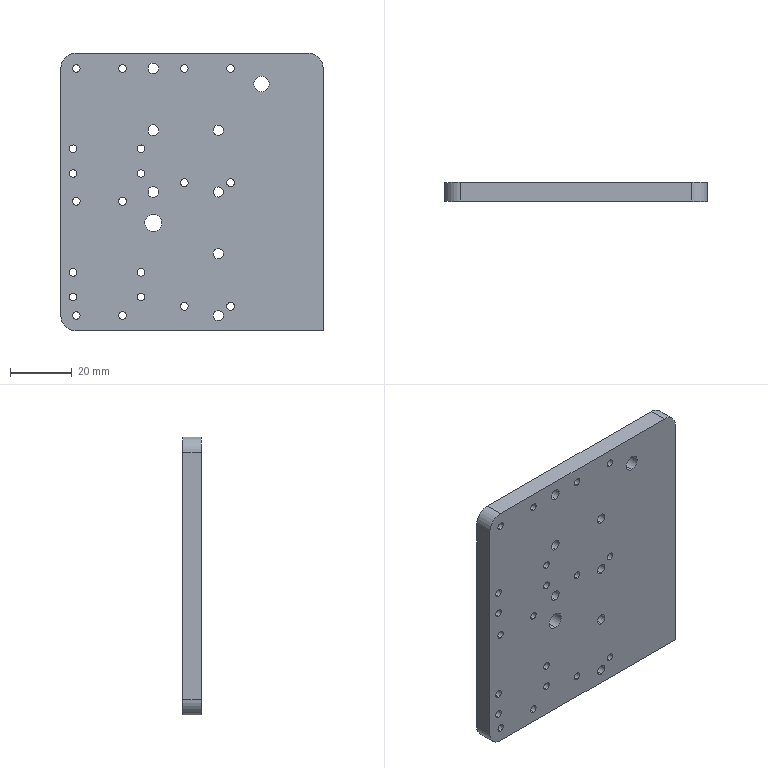Part | STEP file | 0246_201_Plate | 1 solid | 88 faces | box 85 x 6 x 90 mm | volume 44216 mm3 | cylinder 75 | plane 13 | commonest cylinder face diameters 2.5 x48 3.3 x8 3.5 x6 6.5 x6 10 x3 5 x2